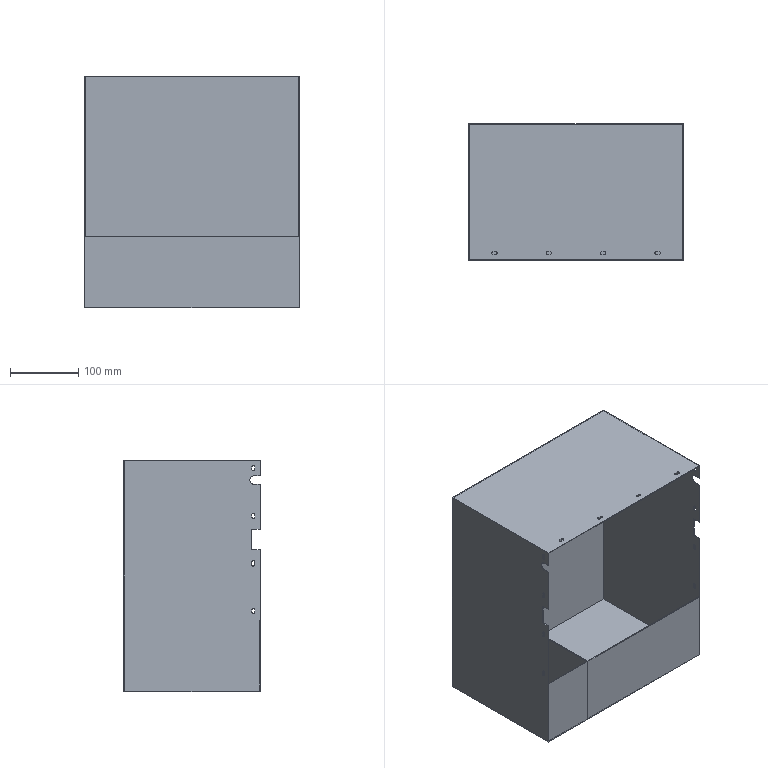Part | STEP file | Lid storage box 001 | 1 solid | 92 faces | box 315 x 200 x 340 mm | volume 428432 mm3 | plane 54 | cylinder 38 | commonest cylinder face diameters 4 x36 12 x2